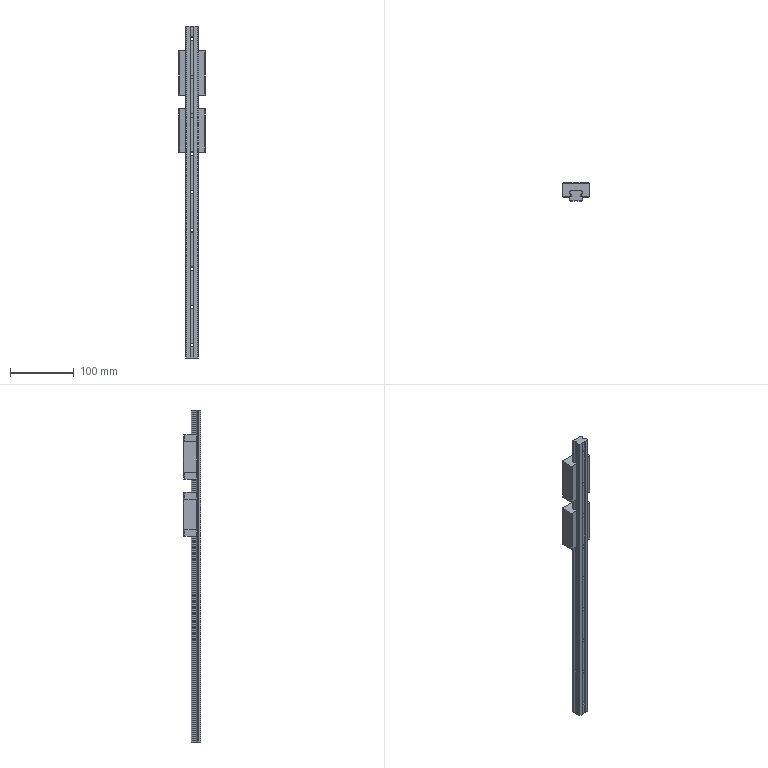Part | NX | features BREP 3 | 3 solids | 433 faces | box 42 x 28 x 520 mm | volume 239515 mm3 | plane 212 | cylinder 197 | cone 24 | commonest cylinder face diameters 1.6 x32 2.5 x24 1 x16 5 x16 3.5 x12 5.5 x12